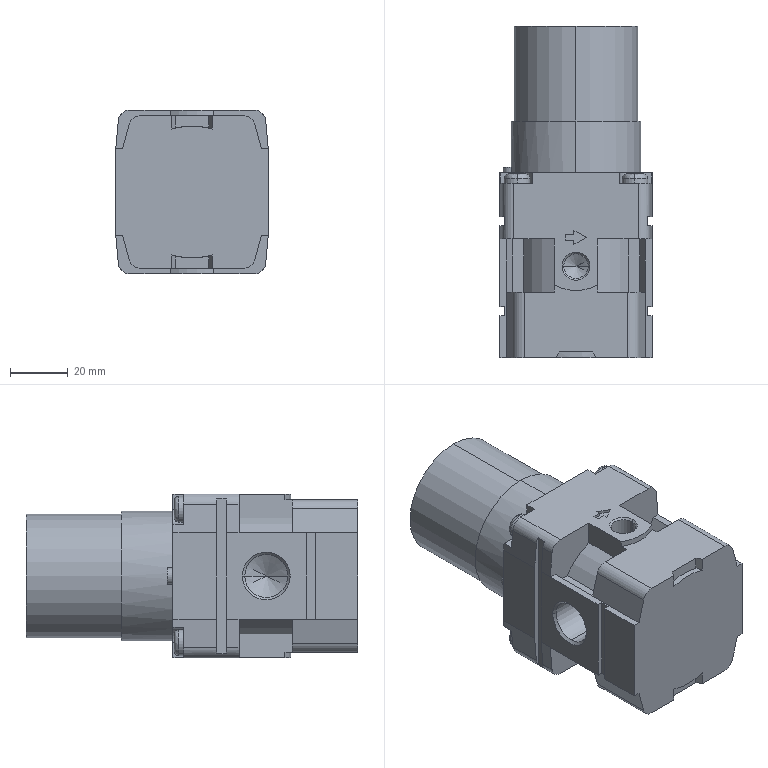Part | STEP file | 11-GY_AW30-03G-A(0)_BODY-30-V10-22111.11 | 1 solid | 174 faces | box 53 x 115.3 x 57 mm | volume 234784 mm3 | plane 111 | cylinder 41 | cone 14 | spline 8 | commonest cylinder face diameters 8 x8 9 x8 43 x6 11 x4 14.95 x4 8.566 x2